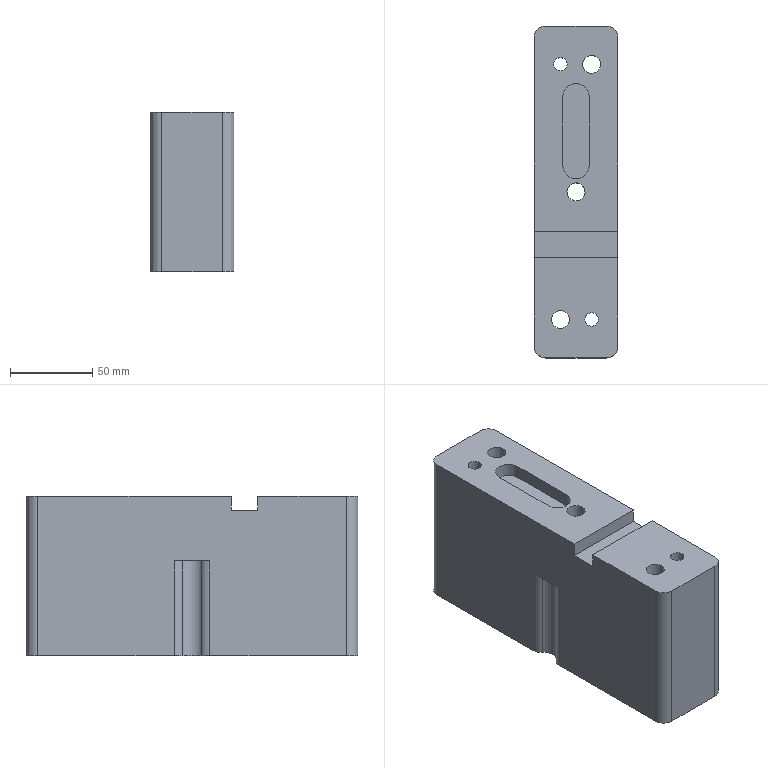Part | STEP file | 1_id150_x_t | 1 solid | 42 faces | box 51 x 202 x 97.035 mm | volume 913093 mm3 | plane 20 | cylinder 20 | cone 2 | commonest cylinder face diameters 12 x4 14 x4 17 x4 11 x3 8.2 x2 16 x2